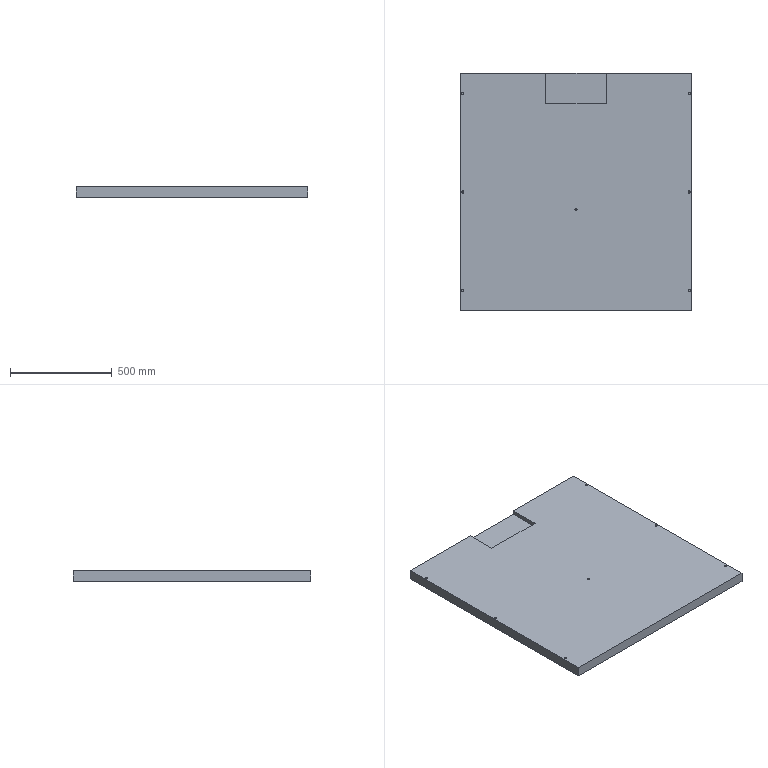Part | 1 solid | 31 faces | box 1140 x 1170 x 50 mm | volume 65777025 mm3 | plane 17 | cylinder 14 | commonest cylinder face diameters 11 x12 10 x2
STEP:
#1=CARTESIAN_POINT('',(-563.,-485.,30.));
#2=VERTEX_POINT('',#1);
#3=CARTESIAN_POINT('',(-552.,-485.,30.));
#4=VERTEX_POINT('',#3);
#5=CARTESIAN_POINT('',(-557.5,-485.,30.));
#6=DIRECTION('',(0.,0.,1.));
#7=DIRECTION('',(-1.,0.,0.));
#8=AXIS2_PLACEMENT_3D('',#5,#6,#7);
#9=CIRCLE('',#8,5.5);
#10=EDGE_CURVE('',#2,#4,#9,.T.);
#11=ORIENTED_EDGE('',*,*,#10,.F.);
#12=CARTESIAN_POINT('',(-563.,-485.,50.));
#13=VERTEX_POINT('',#12);
#14=CARTESIAN_POINT('',(-563.,-485.,30.));
#15=DIRECTION('',(0.,0.,1.));
#16=VECTOR('',#15,1000.);
#17=LINE('',#14,#16);
#18=EDGE_CURVE('',#2,#13,#17,.T.);
#19=ORIENTED_EDGE('',*,*,#18,.T.);
#20=CARTESIAN_POINT('',(-552.,-485.,50.));
#21=VERTEX_POINT('',#20);
#22=CARTESIAN_POINT('',(-557.5,-485.,50.));
#23=DIRECTION('',(0.,0.,1.));
#24=DIRECTION('',(-1.,0.,0.));
#25=AXIS2_PLACEMENT_3D('',#22,#23,#24);
#26=CIRCLE('',#25,5.5);
#27=EDGE_CURVE('',#13,#21,#26,.T.);
#28=ORIENTED_EDGE('',*,*,#27,.T.);
#29=CARTESIAN_POINT('',(-552.,-485.,30.));
#30=DIRECTION('',(0.,0.,1.));
#31=VECTOR('',#30,1000.);
#32=LINE('',#29,#31);
#33=EDGE_CURVE('',#4,#21,#32,.T.);
#34=ORIENTED_EDGE('',*,*,#33,.F.);
#35=EDGE_LOOP('',(#11,#19,#28,#34));
#36=FACE_OUTER_BOUND('',#35,.T.);
#37=CARTESIAN_POINT('',(-557.5,-485.,30.));
#38=DIRECTION('',(0.,0.,1.));
#39=DIRECTION('',(1.,0.,0.));
#40=AXIS2_PLACEMENT_3D('',#37,#38,#39);
#41=CYLINDRICAL_SURFACE('',#40,5.5);
#42=ADVANCED_FACE('',(#36),#41,.F.);
#43=CARTESIAN_POINT('',(-563.,0.,30.));
#44=VERTEX_POINT('',#43);
#45=CARTESIAN_POINT('',(-552.,0.,30.));
#46=VERTEX_POINT('',#45);
#47=CARTESIAN_POINT('',(-557.5,0.,30.));
#48=DIRECTION('',(0.,0.,1.));
#49=DIRECTION('',(-1.,0.,0.));
#50=AXIS2_PLACEMENT_3D('',#47,#48,#49);
#51=CIRCLE('',#50,5.5);
#52=EDGE_CURVE('',#44,#46,#51,.T.);
#53=ORIENTED_EDGE('',*,*,#52,.F.);
#54=CARTESIAN_POINT('',(-563.,0.,50.));
#55=VERTEX_POINT('',#54);
#56=CARTESIAN_POINT('',(-563.,0.,30.));
#57=DIRECTION('',(0.,0.,1.));
#58=VECTOR('',#57,1000.);
#59=LINE('',#56,#58);
#60=EDGE_CURVE('',#44,#55,#59,.T.);
#61=ORIENTED_EDGE('',*,*,#60,.T.);
#62=CARTESIAN_POINT('',(-552.,0.,50.));
#63=VERTEX_POINT('',#62);
#64=CARTESIAN_POINT('',(-557.5,0.,50.));
#65=DIRECTION('',(0.,0.,1.));
#66=DIRECTION('',(-1.,0.,0.));
#67=AXIS2_PLACEMENT_3D('',#64,#65,#66);
#68=CIRCLE('',#67,5.5);
#69=EDGE_CURVE('',#55,#63,#68,.T.);
#70=ORIENTED_EDGE('',*,*,#69,.T.);
#71=CARTESIAN_POINT('',(-552.,0.,30.));
#72=DIRECTION('',(0.,0.,1.));
#73=VECTOR('',#72,1000.);
#74=LINE('',#71,#73);
#75=EDGE_CURVE('',#46,#63,#74,.T.);
#76=ORIENTED_EDGE('',*,*,#75,.F.);
#77=EDGE_LOOP('',(#53,#61,#70,#76));
#78=FACE_OUTER_BOUND('',#77,.T.);
#79=CARTESIAN_POINT('',(-557.5,0.,30.));
#80=DIRECTION('',(0.,0.,1.));
#81=DIRECTION('',(1.,0.,0.));
#82=AXIS2_PLACEMENT_3D('',#79,#80,#81);
#83=CYLINDRICAL_SURFACE('',#82,5.5);
#84=ADVANCED_FACE('',(#78),#83,.F.);
#85=CARTESIAN_POINT('',(-563.,485.,30.));
#86=VERTEX_POINT('',#85);
#87=CARTESIAN_POINT('',(-552.,485.,30.));
#88=VERTEX_POINT('',#87);
#89=CARTESIAN_POINT('',(-557.5,485.,30.));
#90=DIRECTION('',(0.,0.,1.));
#91=DIRECTION('',(-1.,0.,0.));
#92=AXIS2_PLACEMENT_3D('',#89,#90,#91);
#93=CIRCLE('',#92,5.5);
#94=EDGE_CURVE('',#86,#88,#93,.T.);
#95=ORIENTED_EDGE('',*,*,#94,.F.);
#96=CARTESIAN_POINT('',(-563.,485.,50.));
#97=VERTEX_POINT('',#96);
#98=CARTESIAN_POINT('',(-563.,485.,30.));
#99=DIRECTION('',(0.,0.,1.));
#100=VECTOR('',#99,1000.);
#101=LINE('',#98,#100);
#102=EDGE_CURVE('',#86,#97,#101,.T.);
#103=ORIENTED_EDGE('',*,*,#102,.T.);
#104=CARTESIAN_POINT('',(-552.,485.,50.));
#105=VERTEX_POINT('',#104);
#106=CARTESIAN_POINT('',(-557.5,485.,50.));
#107=DIRECTION('',(0.,0.,1.));
#108=DIRECTION('',(-1.,0.,0.));
#109=AXIS2_PLACEMENT_3D('',#106,#107,#108);
#110=CIRCLE('',#109,5.5);
#111=EDGE_CURVE('',#97,#105,#110,.T.);
#112=ORIENTED_EDGE('',*,*,#111,.T.);
#113=CARTESIAN_POINT('',(-552.,485.,30.));
#114=DIRECTION('',(0.,0.,1.));
#115=VECTOR('',#114,1000.);
#116=LINE('',#113,#115);
#117=EDGE_CURVE('',#88,#105,#116,.T.);
#118=ORIENTED_EDGE('',*,*,#117,.F.);
#119=EDGE_LOOP('',(#95,#103,#112,#118));
#120=FACE_OUTER_BOUND('',#119,.T.);
#121=CARTESIAN_POINT('',(-557.5,485.,30.));
#122=DIRECTION('',(0.,0.,1.));
#123=DIRECTION('',(1.,0.,0.));
#124=AXIS2_PLACEMENT_3D('',#121,#122,#123);
#125=CYLINDRICAL_SURFACE('',#124,5.5);
#126=ADVANCED_FACE('',(#120),#125,.F.);
#127=CARTESIAN_POINT('',(552.,485.,30.));
#128=VERTEX_POINT('',#127);
#129=CARTESIAN_POINT('',(563.,485.,30.));
#130=VERTEX_POINT('',#129);
#131=CARTESIAN_POINT('',(557.5,485.,30.));
#132=DIRECTION('',(0.,0.,1.));
#133=DIRECTION('',(1.,0.,0.));
#134=AXIS2_PLACEMENT_3D('',#131,#132,#133);
#135=CIRCLE('',#134,5.5);
#136=EDGE_CURVE('',#128,#130,#135,.T.);
#137=ORIENTED_EDGE('',*,*,#136,.F.);
#138=CARTESIAN_POINT('',(552.,485.,50.));
#139=VERTEX_POINT('',#138);
#140=CARTESIAN_POINT('',(552.,485.,30.));
#141=DIRECTION('',(0.,0.,1.));
#142=VECTOR('',#141,1000.);
#143=LINE('',#140,#142);
#144=EDGE_CURVE('',#128,#139,#143,.T.);
#145=ORIENTED_EDGE('',*,*,#144,.T.);
#146=CARTESIAN_POINT('',(563.,485.,50.));
#147=VERTEX_POINT('',#146);
#148=CARTESIAN_POINT('',(557.5,485.,50.));
#149=DIRECTION('',(0.,0.,1.));
#150=DIRECTION('',(1.,0.,0.));
#151=AXIS2_PLACEMENT_3D('',#148,#149,#150);
#152=CIRCLE('',#151,5.5);
#153=EDGE_CURVE('',#139,#147,#152,.T.);
#154=ORIENTED_EDGE('',*,*,#153,.T.);
#155=CARTESIAN_POINT('',(563.,485.,30.));
#156=DIRECTION('',(0.,0.,1.));
#157=VECTOR('',#156,1000.);
#158=LINE('',#155,#157);
#159=EDGE_CURVE('',#130,#147,#158,.T.);
#160=ORIENTED_EDGE('',*,*,#159,.F.);
#161=EDGE_LOOP('',(#137,#145,#154,#160));
#162=FACE_OUTER_BOUND('',#161,.T.);
#163=CARTESIAN_POINT('',(557.5,485.,30.));
#164=DIRECTION('',(0.,0.,1.));
#165=DIRECTION('',(1.,0.,0.));
#166=AXIS2_PLACEMENT_3D('',#163,#164,#165);
#167=CYLINDRICAL_SURFACE('',#166,5.5);
#168=ADVANCED_FACE('',(#162),#167,.F.);
#169=CARTESIAN_POINT('',(552.,0.,30.));
#170=VERTEX_POINT('',#169);
#171=CARTESIAN_POINT('',(563.,0.,30.));
#172=VERTEX_POINT('',#171);
#173=CARTESIAN_POINT('',(557.5,0.,30.));
#174=DIRECTION('',(0.,0.,1.));
#175=DIRECTION('',(1.,0.,0.));
#176=AXIS2_PLACEMENT_3D('',#173,#174,#175);
#177=CIRCLE('',#176,5.5);
#178=EDGE_CURVE('',#170,#172,#177,.T.);
#179=ORIENTED_EDGE('',*,*,#178,.F.);
#180=CARTESIAN_POINT('',(552.,0.,50.));
#181=VERTEX_POINT('',#180);
#182=CARTESIAN_POINT('',(552.,0.,30.));
#183=DIRECTION('',(0.,0.,1.));
#184=VECTOR('',#183,1000.);
#185=LINE('',#182,#184);
#186=EDGE_CURVE('',#170,#181,#185,.T.);
#187=ORIENTED_EDGE('',*,*,#186,.T.);
#188=CARTESIAN_POINT('',(563.,0.,50.));
#189=VERTEX_POINT('',#188);
#190=CARTESIAN_POINT('',(557.5,0.,50.));
#191=DIRECTION('',(0.,0.,1.));
#192=DIRECTION('',(1.,0.,0.));
#193=AXIS2_PLACEMENT_3D('',#190,#191,#192);
#194=CIRCLE('',#193,5.5);
#195=EDGE_CURVE('',#181,#189,#194,.T.);
#196=ORIENTED_EDGE('',*,*,#195,.T.);
#197=CARTESIAN_POINT('',(563.,0.,30.));
#198=DIRECTION('',(0.,0.,1.));
#199=VECTOR('',#198,1000.);
#200=LINE('',#197,#199);
#201=EDGE_CURVE('',#172,#189,#200,.T.);
#202=ORIENTED_EDGE('',*,*,#201,.F.);
#203=EDGE_LOOP('',(#179,#187,#196,#202));
#204=FACE_OUTER_BOUND('',#203,.T.);
#205=CARTESIAN_POINT('',(557.5,0.,30.));
#206=DIRECTION('',(0.,0.,1.));
#207=DIRECTION('',(1.,0.,0.));
#208=AXIS2_PLACEMENT_3D('',#205,#206,#207);
#209=CYLINDRICAL_SURFACE('',#208,5.5);
#210=ADVANCED_FACE('',(#204),#209,.F.);
#211=CARTESIAN_POINT('',(552.,-485.,30.));
#212=VERTEX_POINT('',#211);
#213=CARTESIAN_POINT('',(563.,-485.,30.));
#214=VERTEX_POINT('',#213);
#215=CARTESIAN_POINT('',(557.5,-485.,30.));
#216=DIRECTION('',(0.,0.,1.));
#217=DIRECTION('',(1.,0.,0.));
#218=AXIS2_PLACEMENT_3D('',#215,#216,#217);
#219=CIRCLE('',#218,5.5);
#220=EDGE_CURVE('',#212,#214,#219,.T.);
#221=ORIENTED_EDGE('',*,*,#220,.F.);
#222=CARTESIAN_POINT('',(552.,-485.,50.));
#223=VERTEX_POINT('',#222);
#224=CARTESIAN_POINT('',(552.,-485.,30.));
#225=DIRECTION('',(0.,0.,1.));
#226=VECTOR('',#225,1000.);
#227=LINE('',#224,#226);
#228=EDGE_CURVE('',#212,#223,#227,.T.);
#229=ORIENTED_EDGE('',*,*,#228,.T.);
#230=CARTESIAN_POINT('',(563.,-485.,50.));
#231=VERTEX_POINT('',#230);
#232=CARTESIAN_POINT('',(557.5,-485.,50.));
#233=DIRECTION('',(0.,0.,1.));
#234=DIRECTION('',(1.,0.,0.));
#235=AXIS2_PLACEMENT_3D('',#232,#233,#234);
#236=CIRCLE('',#235,5.5);
#237=EDGE_CURVE('',#223,#231,#236,.T.);
#238=ORIENTED_EDGE('',*,*,#237,.T.);
#239=CARTESIAN_POINT('',(563.,-485.,30.));
#240=DIRECTION('',(0.,0.,1.));
#241=VECTOR('',#240,1000.);
#242=LINE('',#239,#241);
#243=EDGE_CURVE('',#214,#231,#242,.T.);
#244=ORIENTED_EDGE('',*,*,#243,.F.);
#245=EDGE_LOOP('',(#221,#229,#238,#244));
#246=FACE_OUTER_BOUND('',#245,.T.);
#247=CARTESIAN_POINT('',(557.5,-485.,30.));
#248=DIRECTION('',(0.,0.,1.));
#249=DIRECTION('',(1.,0.,0.));
#250=AXIS2_PLACEMENT_3D('',#247,#248,#249);
#251=CYLINDRICAL_SURFACE('',#250,5.5);
#252=ADVANCED_FACE('',(#246),#251,.F.);
#253=CARTESIAN_POINT('',(-5.,-85.,30.));
#254=VERTEX_POINT('',#253);
#255=CARTESIAN_POINT('',(5.,-85.,30.));
#256=VERTEX_POINT('',#255);
#257=CARTESIAN_POINT('',(0.,-85.,30.));
#258=DIRECTION('',(0.,0.,1.));
#259=DIRECTION('',(1.,0.,0.));
#260=AXIS2_PLACEMENT_3D('',#257,#258,#259);
#261=CIRCLE('',#260,5.);
#262=EDGE_CURVE('',#254,#256,#261,.T.);
#263=ORIENTED_EDGE('',*,*,#262,.F.);
#264=CARTESIAN_POINT('',(-5.,-85.,50.));
#265=VERTEX_POINT('',#264);
#266=CARTESIAN_POINT('',(-5.,-85.,30.));
#267=DIRECTION('',(0.,0.,1.));
#268=VECTOR('',#267,1000.);
#269=LINE('',#266,#268);
#270=EDGE_CURVE('',#254,#265,#269,.T.);
#271=ORIENTED_EDGE('',*,*,#270,.T.);
#272=CARTESIAN_POINT('',(5.,-85.,50.));
#273=VERTEX_POINT('',#272);
#274=CARTESIAN_POINT('',(0.,-85.,50.));
#275=DIRECTION('',(0.,0.,1.));
#276=DIRECTION('',(1.,0.,0.));
#277=AXIS2_PLACEMENT_3D('',#274,#275,#276);
#278=CIRCLE('',#277,5.);
#279=EDGE_CURVE('',#265,#273,#278,.T.);
#280=ORIENTED_EDGE('',*,*,#279,.T.);
#281=CARTESIAN_POINT('',(5.,-85.,30.));
#282=DIRECTION('',(0.,0.,1.));
#283=VECTOR('',#282,1000.);
#284=LINE('',#281,#283);
#285=EDGE_CURVE('',#256,#273,#284,.T.);
#286=ORIENTED_EDGE('',*,*,#285,.F.);
#287=EDGE_LOOP('',(#263,#271,#280,#286));
#288=FACE_OUTER_BOUND('',#287,.T.);
#289=CARTESIAN_POINT('',(0.,-85.,30.));
#290=DIRECTION('',(0.,0.,1.));
#291=DIRECTION('',(1.,0.,0.));
#292=AXIS2_PLACEMENT_3D('',#289,#290,#291);
#293=CYLINDRICAL_SURFACE('',#292,5.);
#294=ADVANCED_FACE('',(#288),#293,.F.);
#295=CARTESIAN_POINT('',(570.,-585.,0.));
#296=VERTEX_POINT('',#295);
#297=CARTESIAN_POINT('',(570.,585.,0.));
#298=VERTEX_POINT('',#297);
#299=CARTESIAN_POINT('',(570.,585.,0.));
#300=DIRECTION('',(0.,1.,0.));
#301=VECTOR('',#300,1000.);
#302=LINE('',#299,#301);
#303=EDGE_CURVE('',#296,#298,#302,.T.);
#304=ORIENTED_EDGE('',*,*,#303,.T.);
#305=CARTESIAN_POINT('',(570.,585.,50.));
#306=VERTEX_POINT('',#305);
#307=CARTESIAN_POINT('',(570.,585.,50.));
#308=DIRECTION('',(0.,0.,-1.));
#309=VECTOR('',#308,1000.);
#310=LINE('',#307,#309);
#311=EDGE_CURVE('',#306,#298,#310,.T.);
#312=ORIENTED_EDGE('',*,*,#311,.F.);
#313=CARTESIAN_POINT('',(570.,-585.,50.));
#314=VERTEX_POINT('',#313);
#315=CARTESIAN_POINT('',(570.,585.,50.));
#316=DIRECTION('',(0.,1.,0.));
#317=VECTOR('',#316,1000.);
#318=LINE('',#315,#317);
#319=EDGE_CURVE('',#314,#306,#318,.T.);
#320=ORIENTED_EDGE('',*,*,#319,.F.);
#321=CARTESIAN_POINT('',(570.,-585.,50.));
#322=DIRECTION('',(0.,0.,-1.));
#323=VECTOR('',#322,1000.);
#324=LINE('',#321,#323);
#325=EDGE_CURVE('',#314,#296,#324,.T.);
#326=ORIENTED_EDGE('',*,*,#325,.T.);
#327=EDGE_LOOP('',(#304,#312,#320,#326));
#328=FACE_OUTER_BOUND('',#327,.T.);
#329=CARTESIAN_POINT('',(570.,585.,50.));
#330=DIRECTION('',(-1.,0.,0.));
#331=DIRECTION('',(0.,-1.,0.));
#332=AXIS2_PLACEMENT_3D('',#329,#330,#331);
#333=PLANE('',#332);
#334=ADVANCED_FACE('',(#328),#333,.F.);
#335=CARTESIAN_POINT('',(150.,585.,30.));
#336=VERTEX_POINT('',#335);
#337=CARTESIAN_POINT('',(-150.,585.,30.));
#338=VERTEX_POINT('',#337);
#339=CARTESIAN_POINT('',(-570.,585.,30.));
#340=DIRECTION('',(-1.,0.,0.));
#341=VECTOR('',#340,1000.);
#342=LINE('',#339,#341);
#343=EDGE_CURVE('',#336,#338,#342,.T.);
#344=ORIENTED_EDGE('',*,*,#343,.F.);
#345=CARTESIAN_POINT('',(150.,585.,50.));
#346=VERTEX_POINT('',#345);
#347=CARTESIAN_POINT('',(150.,585.,50.));
#348=DIRECTION('',(0.,0.,1.));
#349=VECTOR('',#348,1000.);
#350=LINE('',#347,#349);
#351=EDGE_CURVE('',#336,#346,#350,.T.);
#352=ORIENTED_EDGE('',*,*,#351,.T.);
#353=CARTESIAN_POINT('',(-570.,585.,50.));
#354=DIRECTION('',(-1.,0.,0.));
#355=VECTOR('',#354,1000.);
#356=LINE('',#353,#355);
#357=EDGE_CURVE('',#306,#346,#356,.T.);
#358=ORIENTED_EDGE('',*,*,#357,.F.);
#359=ORIENTED_EDGE('',*,*,#311,.T.);
#360=CARTESIAN_POINT('',(-570.,585.,0.));
#361=VERTEX_POINT('',#360);
#362=CARTESIAN_POINT('',(-570.,585.,0.));
#363=DIRECTION('',(-1.,0.,0.));
#364=VECTOR('',#363,1000.);
#365=LINE('',#362,#364);
#366=EDGE_CURVE('',#298,#361,#365,.T.);
#367=ORIENTED_EDGE('',*,*,#366,.T.);
#368=CARTESIAN_POINT('',(-570.,585.,50.));
#369=VERTEX_POINT('',#368);
#370=CARTESIAN_POINT('',(-570.,585.,50.));
#371=DIRECTION('',(0.,0.,-1.));
#372=VECTOR('',#371,1000.);
#373=LINE('',#370,#372);
#374=EDGE_CURVE('',#369,#361,#373,.T.);
#375=ORIENTED_EDGE('',*,*,#374,.F.);
#376=CARTESIAN_POINT('',(-150.,585.,50.));
#377=VERTEX_POINT('',#376);
#378=CARTESIAN_POINT('',(-570.,585.,50.));
#379=DIRECTION('',(-1.,0.,0.));
#380=VECTOR('',#379,1000.);
#381=LINE('',#378,#380);
#382=EDGE_CURVE('',#377,#369,#381,.T.);
#383=ORIENTED_EDGE('',*,*,#382,.F.);
#384=CARTESIAN_POINT('',(-150.,585.,50.));
#385=DIRECTION('',(0.,0.,-1.));
#386=VECTOR('',#385,1000.);
#387=LINE('',#384,#386);
#388=EDGE_CURVE('',#377,#338,#387,.T.);
#389=ORIENTED_EDGE('',*,*,#388,.T.);
#390=EDGE_LOOP('',(#344,#352,#358,#359,#367,#375,#383,#389));
#391=FACE_OUTER_BOUND('',#390,.T.);
#392=CARTESIAN_POINT('',(-570.,585.,50.));
#393=DIRECTION('',(0.,-1.,0.));
#394=DIRECTION('',(0.,0.,-1.));
#395=AXIS2_PLACEMENT_3D('',#392,#393,#394);
#396=PLANE('',#395);
#397=ADVANCED_FACE('',(#391),#396,.F.);
#398=CARTESIAN_POINT('',(-570.,-585.,0.));
#399=VERTEX_POINT('',#398);
#400=CARTESIAN_POINT('',(-570.,585.,0.));
#401=DIRECTION('',(0.,-1.,0.));
#402=VECTOR('',#401,1000.);
#403=LINE('',#400,#402);
#404=EDGE_CURVE('',#361,#399,#403,.T.);
#405=ORIENTED_EDGE('',*,*,#404,.T.);
#406=CARTESIAN_POINT('',(-570.,-585.,50.));
#407=VERTEX_POINT('',#406);
#408=CARTESIAN_POINT('',(-570.,-585.,50.));
#409=DIRECTION('',(0.,0.,-1.));
#410=VECTOR('',#409,1000.);
#411=LINE('',#408,#410);
#412=EDGE_CURVE('',#407,#399,#411,.T.);
#413=ORIENTED_EDGE('',*,*,#412,.F.);
#414=CARTESIAN_POINT('',(-570.,585.,50.));
#415=DIRECTION('',(0.,-1.,0.));
#416=VECTOR('',#415,1000.);
#417=LINE('',#414,#416);
#418=EDGE_CURVE('',#369,#407,#417,.T.);
#419=ORIENTED_EDGE('',*,*,#418,.F.);
#420=ORIENTED_EDGE('',*,*,#374,.T.);
#421=EDGE_LOOP('',(#405,#413,#419,#420));
#422=FACE_OUTER_BOUND('',#421,.T.);
#423=CARTESIAN_POINT('',(-570.,585.,50.));
#424=DIRECTION('',(1.,0.,0.));
#425=DIRECTION('',(0.,1.,0.));
#426=AXIS2_PLACEMENT_3D('',#423,#424,#425);
#427=PLANE('',#426);
#428=ADVANCED_FACE('',(#422),#427,.F.);
#429=CARTESIAN_POINT('',(-570.,-585.,0.));
#430=DIRECTION('',(1.,0.,0.));
#431=VECTOR('',#430,1000.);
#432=LINE('',#429,#431);
#433=EDGE_CURVE('',#399,#296,#432,.T.);
#434=ORIENTED_EDGE('',*,*,#433,.T.);
#435=ORIENTED_EDGE('',*,*,#325,.F.);
#436=CARTESIAN_POINT('',(-570.,-585.,50.));
#437=DIRECTION('',(1.,0.,0.));
#438=VECTOR('',#437,1000.);
#439=LINE('',#436,#438);
#440=EDGE_CURVE('',#407,#314,#439,.T.);
#441=ORIENTED_EDGE('',*,*,#440,.F.);
#442=ORIENTED_EDGE('',*,*,#412,.T.);
#443=EDGE_LOOP('',(#434,#435,#441,#442));
#444=FACE_OUTER_BOUND('',#443,.T.);
#445=CARTESIAN_POINT('',(-570.,-585.,50.));
#446=DIRECTION('',(0.,1.,0.));
#447=DIRECTION('',(0.,0.,1.));
#448=AXIS2_PLACEMENT_3D('',#445,#446,#447);
#449=PLANE('',#448);
#450=ADVANCED_FACE('',(#444),#449,.F.);
#451=CARTESIAN_POINT('',(-557.5,-485.,50.));
#452=DIRECTION('',(0.,0.,1.));
#453=DIRECTION('',(-1.,0.,0.));
#454=AXIS2_PLACEMENT_3D('',#451,#452,#453);
#455=CIRCLE('',#454,5.5);
#456=EDGE_CURVE('',#21,#13,#455,.T.);
#457=ORIENTED_EDGE('',*,*,#456,.F.);
#458=ORIENTED_EDGE('',*,*,#27,.F.);
#459=EDGE_LOOP('',(#457,#458));
#460=FACE_BOUND('',#459,.T.);
#461=CARTESIAN_POINT('',(-557.5,0.,50.));
#462=DIRECTION('',(0.,0.,1.));
#463=DIRECTION('',(-1.,0.,0.));
#464=AXIS2_PLACEMENT_3D('',#461,#462,#463);
#465=CIRCLE('',#464,5.5);
#466=EDGE_CURVE('',#63,#55,#465,.T.);
#467=ORIENTED_EDGE('',*,*,#466,.F.);
#468=ORIENTED_EDGE('',*,*,#69,.F.);
#469=EDGE_LOOP('',(#467,#468));
#470=FACE_BOUND('',#469,.T.);
#471=CARTESIAN_POINT('',(-557.5,485.,50.));
#472=DIRECTION('',(0.,0.,1.));
#473=DIRECTION('',(-1.,0.,0.));
#474=AXIS2_PLACEMENT_3D('',#471,#472,#473);
#475=CIRCLE('',#474,5.5);
#476=EDGE_CURVE('',#105,#97,#475,.T.);
#477=ORIENTED_EDGE('',*,*,#476,.F.);
#478=ORIENTED_EDGE('',*,*,#111,.F.);
#479=EDGE_LOOP('',(#477,#478));
#480=FACE_BOUND('',#479,.T.);
#481=CARTESIAN_POINT('',(557.5,485.,50.));
#482=DIRECTION('',(0.,0.,1.));
#483=DIRECTION('',(1.,0.,0.));
#484=AXIS2_PLACEMENT_3D('',#481,#482,#483);
#485=CIRCLE('',#484,5.5);
#486=EDGE_CURVE('',#147,#139,#485,.T.);
#487=ORIENTED_EDGE('',*,*,#486,.F.);
#488=ORIENTED_EDGE('',*,*,#153,.F.);
#489=EDGE_LOOP('',(#487,#488));
#490=FACE_BOUND('',#489,.T.);
#491=CARTESIAN_POINT('',(557.5,0.,50.));
#492=DIRECTION('',(0.,0.,1.));
#493=DIRECTION('',(1.,0.,0.));
#494=AXIS2_PLACEMENT_3D('',#491,#492,#493);
#495=CIRCLE('',#494,5.5);
#496=EDGE_CURVE('',#189,#181,#495,.T.);
#497=ORIENTED_EDGE('',*,*,#496,.F.);
#498=ORIENTED_EDGE('',*,*,#195,.F.);
#499=EDGE_LOOP('',(#497,#498));
#500=FACE_BOUND('',#499,.T.);
#501=CARTESIAN_POINT('',(557.5,-485.,50.));
#502=DIRECTION('',(0.,0.,1.));
#503=DIRECTION('',(1.,0.,0.));
#504=AXIS2_PLACEMENT_3D('',#501,#502,#503);
#505=CIRCLE('',#504,5.5);
#506=EDGE_CURVE('',#231,#223,#505,.T.);
#507=ORIENTED_EDGE('',*,*,#506,.F.);
#508=ORIENTED_EDGE('',*,*,#237,.F.);
#509=EDGE_LOOP('',(#507,#508));
#510=FACE_BOUND('',#509,.T.);
#511=CARTESIAN_POINT('',(0.,-85.,50.));
#512=DIRECTION('',(0.,0.,1.));
#513=DIRECTION('',(1.,0.,0.));
#514=AXIS2_PLACEMENT_3D('',#511,#512,#513);
#515=CIRCLE('',#514,5.);
#516=EDGE_CURVE('',#273,#265,#515,.T.);
#517=ORIENTED_EDGE('',*,*,#516,.F.);
#518=ORIENTED_EDGE('',*,*,#279,.F.);
#519=EDGE_LOOP('',(#517,#518));
#520=FACE_BOUND('',#519,.T.);
#521=CARTESIAN_POINT('',(150.,435.,50.));
#522=VERTEX_POINT('',#521);
#523=CARTESIAN_POINT('',(150.,735.,50.));
#524=DIRECTION('',(0.,1.,0.));
#525=VECTOR('',#524,1000.);
#526=LINE('',#523,#525);
#527=EDGE_CURVE('',#522,#346,#526,.T.);
#528=ORIENTED_EDGE('',*,*,#527,.F.);
#529=CARTESIAN_POINT('',(-150.,435.,50.));
#530=VERTEX_POINT('',#529);
#531=CARTESIAN_POINT('',(-150.,435.,50.));
#532=DIRECTION('',(1.,0.,0.));
#533=VECTOR('',#532,1000.);
#534=LINE('',#531,#533);
#535=EDGE_CURVE('',#530,#522,#534,.T.);
#536=ORIENTED_EDGE('',*,*,#535,.F.);
#537=CARTESIAN_POINT('',(-150.,0.,50.));
#538=DIRECTION('',(0.,-1.,0.));
#539=VECTOR('',#538,1000.);
#540=LINE('',#537,#539);
#541=EDGE_CURVE('',#377,#530,#540,.T.);
#542=ORIENTED_EDGE('',*,*,#541,.F.);
#543=ORIENTED_EDGE('',*,*,#382,.T.);
#544=ORIENTED_EDGE('',*,*,#418,.T.);
#545=ORIENTED_EDGE('',*,*,#440,.T.);
#546=ORIENTED_EDGE('',*,*,#319,.T.);
#547=ORIENTED_EDGE('',*,*,#357,.T.);
#548=EDGE_LOOP('',(#528,#536,#542,#543,#544,#545,#546,#547));
#549=FACE_OUTER_BOUND('',#548,.T.);
#550=CARTESIAN_POINT('',(0.,0.,50.));
#551=DIRECTION('',(0.,0.,1.));
#552=DIRECTION('',(1.,0.,0.));
#553=AXIS2_PLACEMENT_3D('',#550,#551,#552);
#554=PLANE('',#553);
#555=ADVANCED_FACE('',(#460,#470,#480,#490,#500,#510,#520,#549),#554,.T.);
#556=ORIENTED_EDGE('',*,*,#303,.F.);
#557=ORIENTED_EDGE('',*,*,#433,.F.);
#558=ORIENTED_EDGE('',*,*,#404,.F.);
#559=ORIENTED_EDGE('',*,*,#366,.F.);
#560=EDGE_LOOP('',(#556,#557,#558,#559));
#561=FACE_OUTER_BOUND('',#560,.T.);
#562=CARTESIAN_POINT('',(0.,0.,0.));
#563=DIRECTION('',(0.,0.,1.));
#564=DIRECTION('',(1.,0.,0.));
#565=AXIS2_PLACEMENT_3D('',#562,#563,#564);
#566=PLANE('',#565);
#567=ADVANCED_FACE('',(#561),#566,.F.);
#568=ORIENTED_EDGE('',*,*,#343,.T.);
#569=CARTESIAN_POINT('',(-150.,435.,30.));
#570=VERTEX_POINT('',#569);
#571=CARTESIAN_POINT('',(-150.,735.,30.));
#572=DIRECTION('',(0.,-1.,0.));
#573=VECTOR('',#572,1000.);
#574=LINE('',#571,#573);
#575=EDGE_CURVE('',#338,#570,#574,.T.);
#576=ORIENTED_EDGE('',*,*,#575,.T.);
#577=CARTESIAN_POINT('',(150.,435.,30.));
#578=VERTEX_POINT('',#577);
#579=CARTESIAN_POINT('',(-150.,435.,30.));
#580=DIRECTION('',(1.,0.,0.));
#581=VECTOR('',#580,1000.);
#582=LINE('',#579,#581);
#583=EDGE_CURVE('',#570,#578,#582,.T.);
#584=ORIENTED_EDGE('',*,*,#583,.T.);
#585=CARTESIAN_POINT('',(150.,735.,30.));
#586=DIRECTION('',(0.,1.,0.));
#587=VECTOR('',#586,1000.);
#588=LINE('',#585,#587);
#589=EDGE_CURVE('',#578,#336,#588,.T.);
#590=ORIENTED_EDGE('',*,*,#589,.T.);
#591=EDGE_LOOP('',(#568,#576,#584,#590));
#592=FACE_OUTER_BOUND('',#591,.T.);
#593=CARTESIAN_POINT('',(0.,0.,30.));
#594=DIRECTION('',(0.,0.,1.));
#595=DIRECTION('',(1.,0.,0.));
#596=AXIS2_PLACEMENT_3D('',#593,#594,#595);
#597=PLANE('',#596);
#598=ADVANCED_FACE('',(#592),#597,.T.);
#599=ORIENTED_EDGE('',*,*,#589,.F.);
#600=CARTESIAN_POINT('',(150.,435.,30.));
#601=DIRECTION('',(0.,0.,1.));
#602=VECTOR('',#601,1000.);
#603=LINE('',#600,#602);
#604=EDGE_CURVE('',#578,#522,#603,.T.);
#605=ORIENTED_EDGE('',*,*,#604,.T.);
#606=ORIENTED_EDGE('',*,*,#527,.T.);
#607=ORIENTED_EDGE('',*,*,#351,.F.);
#608=EDGE_LOOP('',(#599,#605,#606,#607));
#609=FACE_OUTER_BOUND('',#608,.T.);
#610=CARTESIAN_POINT('',(150.,735.,30.));
#611=DIRECTION('',(1.,0.,0.));
#612=DIRECTION('',(0.,1.,0.));
#613=AXIS2_PLACEMENT_3D('',#610,#611,#612);
#614=PLANE('',#613);
#615=ADVANCED_FACE('',(#609),#614,.F.);
#616=ORIENTED_EDGE('',*,*,#541,.T.);
#617=CARTESIAN_POINT('',(-150.,435.,30.));
#618=DIRECTION('',(0.,0.,1.));
#619=VECTOR('',#618,1000.);
#620=LINE('',#617,#619);
#621=EDGE_CURVE('',#570,#530,#620,.T.);
#622=ORIENTED_EDGE('',*,*,#621,.F.);
#623=ORIENTED_EDGE('',*,*,#575,.F.);
#624=ORIENTED_EDGE('',*,*,#388,.F.);
#625=EDGE_LOOP('',(#616,#622,#623,#624));
#626=FACE_OUTER_BOUND('',#625,.T.);
#627=CARTESIAN_POINT('',(-150.,735.,30.));
#628=DIRECTION('',(-1.,0.,0.));
#629=DIRECTION('',(0.,-1.,0.));
#630=AXIS2_PLACEMENT_3D('',#627,#628,#629);
#631=PLANE('',#630);
#632=ADVANCED_FACE('',(#626),#631,.F.);
#633=ORIENTED_EDGE('',*,*,#535,.T.);
#634=ORIENTED_EDGE('',*,*,#604,.F.);
#635=ORIENTED_EDGE('',*,*,#583,.F.);
#636=ORIENTED_EDGE('',*,*,#621,.T.);
#637=EDGE_LOOP('',(#633,#634,#635,#636));
#638=FACE_OUTER_BOUND('',#637,.T.);
#639=CARTESIAN_POINT('',(-150.,435.,30.));
#640=DIRECTION('',(0.,-1.,0.));
#641=DIRECTION('',(0.,0.,-1.));
#642=AXIS2_PLACEMENT_3D('',#639,#640,#641);
#643=PLANE('',#642);
#644=ADVANCED_FACE('',(#638),#643,.F.);
#645=ORIENTED_EDGE('',*,*,#270,.F.);
#646=CARTESIAN_POINT('',(0.,-85.,30.));
#647=DIRECTION('',(0.,0.,1.));
#648=DIRECTION('',(1.,0.,0.));
#649=AXIS2_PLACEMENT_3D('',#646,#647,#648);
#650=CIRCLE('',#649,5.);
#651=EDGE_CURVE('',#256,#254,#650,.T.);
#652=ORIENTED_EDGE('',*,*,#651,.F.);
#653=ORIENTED_EDGE('',*,*,#285,.T.);
#654=ORIENTED_EDGE('',*,*,#516,.T.);
#655=EDGE_LOOP('',(#645,#652,#653,#654));
#656=FACE_OUTER_BOUND('',#655,.T.);
#657=CARTESIAN_POINT('',(0.,-85.,30.));
#658=DIRECTION('',(0.,0.,1.));
#659=DIRECTION('',(1.,0.,0.));
#660=AXIS2_PLACEMENT_3D('',#657,#658,#659);
#661=CYLINDRICAL_SURFACE('',#660,5.);
#662=ADVANCED_FACE('',(#656),#661,.F.);
#663=ORIENTED_EDGE('',*,*,#651,.T.);
#664=ORIENTED_EDGE('',*,*,#262,.T.);
#665=EDGE_LOOP('',(#663,#664));
#666=FACE_OUTER_BOUND('',#665,.T.);
#667=CARTESIAN_POINT('',(0.,-85.,30.));
#668=DIRECTION('',(0.,0.,1.));
#669=DIRECTION('',(1.,0.,0.));
#670=AXIS2_PLACEMENT_3D('',#667,#668,#669);
#671=PLANE('',#670);
#672=ADVANCED_FACE('',(#666),#671,.T.);
#673=ORIENTED_EDGE('',*,*,#228,.F.);
#674=CARTESIAN_POINT('',(557.5,-485.,30.));
#675=DIRECTION('',(0.,0.,1.));
#676=DIRECTION('',(1.,0.,0.));
#677=AXIS2_PLACEMENT_3D('',#674,#675,#676);
#678=CIRCLE('',#677,5.5);
#679=EDGE_CURVE('',#214,#212,#678,.T.);
#680=ORIENTED_EDGE('',*,*,#679,.F.);
#681=ORIENTED_EDGE('',*,*,#243,.T.);
#682=ORIENTED_EDGE('',*,*,#506,.T.);
#683=EDGE_LOOP('',(#673,#680,#681,#682));
#684=FACE_OUTER_BOUND('',#683,.T.);
#685=CARTESIAN_POINT('',(557.5,-485.,30.));
#686=DIRECTION('',(0.,0.,1.));
#687=DIRECTION('',(1.,0.,0.));
#688=AXIS2_PLACEMENT_3D('',#685,#686,#687);
#689=CYLINDRICAL_SURFACE('',#688,5.5);
#690=ADVANCED_FACE('',(#684),#689,.F.);
#691=ORIENTED_EDGE('',*,*,#679,.T.);
#692=ORIENTED_EDGE('',*,*,#220,.T.);
#693=EDGE_LOOP('',(#691,#692));
#694=FACE_OUTER_BOUND('',#693,.T.);
#695=CARTESIAN_POINT('',(557.5,-485.,30.));
#696=DIRECTION('',(0.,0.,1.));
#697=DIRECTION('',(1.,0.,0.));
#698=AXIS2_PLACEMENT_3D('',#695,#696,#697);
#699=PLANE('',#698);
#700=ADVANCED_FACE('',(#694),#699,.T.);
#701=ORIENTED_EDGE('',*,*,#186,.F.);
#702=CARTESIAN_POINT('',(557.5,0.,30.));
#703=DIRECTION('',(0.,0.,1.));
#704=DIRECTION('',(1.,0.,0.));
#705=AXIS2_PLACEMENT_3D('',#702,#703,#704);
#706=CIRCLE('',#705,5.5);
#707=EDGE_CURVE('',#172,#170,#706,.T.);
#708=ORIENTED_EDGE('',*,*,#707,.F.);
#709=ORIENTED_EDGE('',*,*,#201,.T.);
#710=ORIENTED_EDGE('',*,*,#496,.T.);
#711=EDGE_LOOP('',(#701,#708,#709,#710));
#712=FACE_OUTER_BOUND('',#711,.T.);
#713=CARTESIAN_POINT('',(557.5,0.,30.));
#714=DIRECTION('',(0.,0.,1.));
#715=DIRECTION('',(1.,0.,0.));
#716=AXIS2_PLACEMENT_3D('',#713,#714,#715);
#717=CYLINDRICAL_SURFACE('',#716,5.5);
#718=ADVANCED_FACE('',(#712),#717,.F.);
#719=ORIENTED_EDGE('',*,*,#707,.T.);
#720=ORIENTED_EDGE('',*,*,#178,.T.);
#721=EDGE_LOOP('',(#719,#720));
#722=FACE_OUTER_BOUND('',#721,.T.);
#723=CARTESIAN_POINT('',(557.5,0.,30.));
#724=DIRECTION('',(0.,0.,1.));
#725=DIRECTION('',(1.,0.,0.));
#726=AXIS2_PLACEMENT_3D('',#723,#724,#725);
#727=PLANE('',#726);
#728=ADVANCED_FACE('',(#722),#727,.T.);
#729=ORIENTED_EDGE('',*,*,#144,.F.);
#730=CARTESIAN_POINT('',(557.5,485.,30.));
#731=DIRECTION('',(0.,0.,1.));
#732=DIRECTION('',(1.,0.,0.));
#733=AXIS2_PLACEMENT_3D('',#730,#731,#732);
#734=CIRCLE('',#733,5.5);
#735=EDGE_CURVE('',#130,#128,#734,.T.);
#736=ORIENTED_EDGE('',*,*,#735,.F.);
#737=ORIENTED_EDGE('',*,*,#159,.T.);
#738=ORIENTED_EDGE('',*,*,#486,.T.);
#739=EDGE_LOOP('',(#729,#736,#737,#738));
#740=FACE_OUTER_BOUND('',#739,.T.);
#741=CARTESIAN_POINT('',(557.5,485.,30.));
#742=DIRECTION('',(0.,0.,1.));
#743=DIRECTION('',(1.,0.,0.));
#744=AXIS2_PLACEMENT_3D('',#741,#742,#743);
#745=CYLINDRICAL_SURFACE('',#744,5.5);
#746=ADVANCED_FACE('',(#740),#745,.F.);
#747=ORIENTED_EDGE('',*,*,#735,.T.);
#748=ORIENTED_EDGE('',*,*,#136,.T.);
#749=EDGE_LOOP('',(#747,#748));
#750=FACE_OUTER_BOUND('',#749,.T.);
#751=CARTESIAN_POINT('',(557.5,485.,30.));
#752=DIRECTION('',(0.,0.,1.));
#753=DIRECTION('',(1.,0.,0.));
#754=AXIS2_PLACEMENT_3D('',#751,#752,#753);
#755=PLANE('',#754);
#756=ADVANCED_FACE('',(#750),#755,.T.);
#757=ORIENTED_EDGE('',*,*,#102,.F.);
#758=CARTESIAN_POINT('',(-557.5,485.,30.));
#759=DIRECTION('',(0.,0.,1.));
#760=DIRECTION('',(-1.,0.,0.));
#761=AXIS2_PLACEMENT_3D('',#758,#759,#760);
#762=CIRCLE('',#761,5.5);
#763=EDGE_CURVE('',#88,#86,#762,.T.);
#764=ORIENTED_EDGE('',*,*,#763,.F.);
#765=ORIENTED_EDGE('',*,*,#117,.T.);
#766=ORIENTED_EDGE('',*,*,#476,.T.);
#767=EDGE_LOOP('',(#757,#764,#765,#766));
#768=FACE_OUTER_BOUND('',#767,.T.);
#769=CARTESIAN_POINT('',(-557.5,485.,30.));
#770=DIRECTION('',(0.,0.,1.));
#771=DIRECTION('',(1.,0.,0.));
#772=AXIS2_PLACEMENT_3D('',#769,#770,#771);
#773=CYLINDRICAL_SURFACE('',#772,5.5);
#774=ADVANCED_FACE('',(#768),#773,.F.);
#775=ORIENTED_EDGE('',*,*,#763,.T.);
#776=ORIENTED_EDGE('',*,*,#94,.T.);
#777=EDGE_LOOP('',(#775,#776));
#778=FACE_OUTER_BOUND('',#777,.T.);
#779=CARTESIAN_POINT('',(-557.5,485.,30.));
#780=DIRECTION('',(0.,0.,-1.));
#781=DIRECTION('',(-1.,0.,0.));
#782=AXIS2_PLACEMENT_3D('',#779,#780,#781);
#783=PLANE('',#782);
#784=ADVANCED_FACE('',(#778),#783,.F.);
#785=ORIENTED_EDGE('',*,*,#60,.F.);
#786=CARTESIAN_POINT('',(-557.5,0.,30.));
#787=DIRECTION('',(0.,0.,1.));
#788=DIRECTION('',(-1.,0.,0.));
#789=AXIS2_PLACEMENT_3D('',#786,#787,#788);
#790=CIRCLE('',#789,5.5);
#791=EDGE_CURVE('',#46,#44,#790,.T.);
#792=ORIENTED_EDGE('',*,*,#791,.F.);
#793=ORIENTED_EDGE('',*,*,#75,.T.);
#794=ORIENTED_EDGE('',*,*,#466,.T.);
#795=EDGE_LOOP('',(#785,#792,#793,#794));
#796=FACE_OUTER_BOUND('',#795,.T.);
#797=CARTESIAN_POINT('',(-557.5,0.,30.));
#798=DIRECTION('',(0.,0.,1.));
#799=DIRECTION('',(1.,0.,0.));
#800=AXIS2_PLACEMENT_3D('',#797,#798,#799);
#801=CYLINDRICAL_SURFACE('',#800,5.5);
#802=ADVANCED_FACE('',(#796),#801,.F.);
#803=ORIENTED_EDGE('',*,*,#791,.T.);
#804=ORIENTED_EDGE('',*,*,#52,.T.);
#805=EDGE_LOOP('',(#803,#804));
#806=FACE_OUTER_BOUND('',#805,.T.);
#807=CARTESIAN_POINT('',(-557.5,0.,30.));
#808=DIRECTION('',(0.,0.,-1.));
#809=DIRECTION('',(-1.,0.,0.));
#810=AXIS2_PLACEMENT_3D('',#807,#808,#809);
#811=PLANE('',#810);
#812=ADVANCED_FACE('',(#806),#811,.F.);
#813=ORIENTED_EDGE('',*,*,#18,.F.);
#814=CARTESIAN_POINT('',(-557.5,-485.,30.));
#815=DIRECTION('',(0.,0.,1.));
#816=DIRECTION('',(-1.,0.,0.));
#817=AXIS2_PLACEMENT_3D('',#814,#815,#816);
#818=CIRCLE('',#817,5.5);
#819=EDGE_CURVE('',#4,#2,#818,.T.);
#820=ORIENTED_EDGE('',*,*,#819,.F.);
#821=ORIENTED_EDGE('',*,*,#33,.T.);
#822=ORIENTED_EDGE('',*,*,#456,.T.);
#823=EDGE_LOOP('',(#813,#820,#821,#822));
#824=FACE_OUTER_BOUND('',#823,.T.);
#825=CARTESIAN_POINT('',(-557.5,-485.,30.));
#826=DIRECTION('',(0.,0.,1.));
#827=DIRECTION('',(1.,0.,0.));
#828=AXIS2_PLACEMENT_3D('',#825,#826,#827);
#829=CYLINDRICAL_SURFACE('',#828,5.5);
#830=ADVANCED_FACE('',(#824),#829,.F.);
#831=ORIENTED_EDGE('',*,*,#819,.T.);
#832=ORIENTED_EDGE('',*,*,#10,.T.);
#833=EDGE_LOOP('',(#831,#832));
#834=FACE_OUTER_BOUND('',#833,.T.);
#835=CARTESIAN_POINT('',(-557.5,-485.,30.));
#836=DIRECTION('',(0.,0.,-1.));
#837=DIRECTION('',(-1.,0.,0.));
#838=AXIS2_PLACEMENT_3D('',#835,#836,#837);
#839=PLANE('',#838);
#840=ADVANCED_FACE('',(#834),#839,.F.);
#841=CLOSED_SHELL('',(#42,#84,#126,#168,#210,#252,#294,#334,#397,#428,#450,#555,#567,#598,#615,#632,#644,#662,#672,#690,#700,#718,#728,#746,#756,#774,#784,#802,#812,#830,#840));
#842=MANIFOLD_SOLID_BREP('',#841);
#843=CARTESIAN_POINT('',(0.,0.,0.));
#844=DIRECTION('',(0.,0.,1.));
#845=DIRECTION('',(1.,0.,0.));
#846=AXIS2_PLACEMENT_3D('',#843,#844,#845);
#847=(LENGTH_UNIT()NAMED_UNIT(*)SI_UNIT(.MILLI.,.METRE.));
#848=UNCERTAINTY_MEASURE_WITH_UNIT(LENGTH_MEASURE(0.00001),#847,'','');
#849=(NAMED_UNIT(*)PLANE_ANGLE_UNIT()SI_UNIT($,.RADIAN.));
#850=(NAMED_UNIT(*)SI_UNIT($,.STERADIAN.)SOLID_ANGLE_UNIT());
#851=(GEOMETRIC_REPRESENTATION_CONTEXT(3)GLOBAL_UNCERTAINTY_ASSIGNED_CONTEXT((#848))GLOBAL_UNIT_ASSIGNED_CONTEXT((#847,#849,#850))REPRESENTATION_CONTEXT('',''));
#852=ADVANCED_BREP_SHAPE_REPRESENTATION('',(#842,#846),#851);